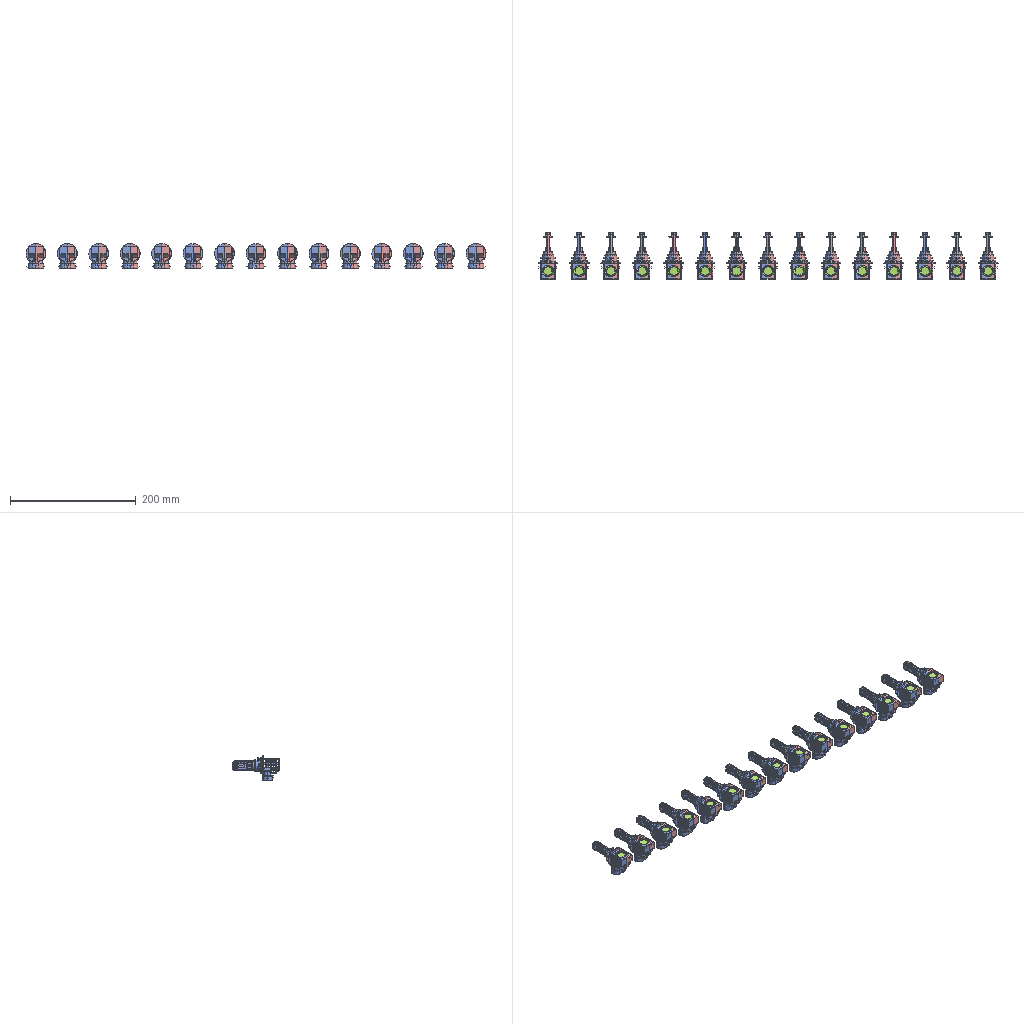Assembly | SolidWorks | 7 different items | 120 placed | box 731 x 74 x 39 mm
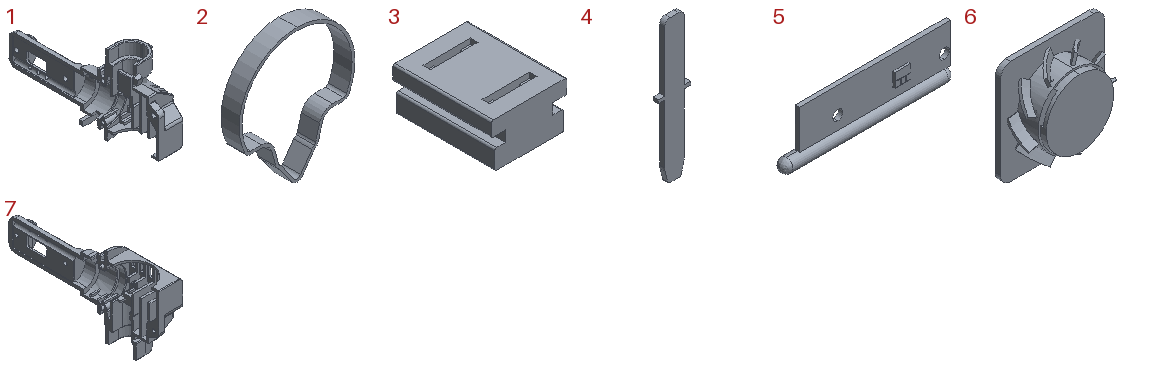Parts list (item | quantity | size | volume | features):
1 | x15 | 19.75 x 73.802 x 39.25 mm | 4726 mm3 | features ICE 12, MoveFace 5, BaseBody 1, Chamfer 1
2 | x15 | 16 x 2.5 x 18.5 mm | 53.347 mm3 | features BaseBody 1
3 | x15 | 7.7 x 10 x 4.6 mm | 286.602 mm3 | features BaseBody 1
4 | x30 | 4.8 x 0.75 x 21 mm | 45.412 mm3 | features BaseBody 1
5 | x15 | 37.94 x 3 x 11.75 mm | 563.627 mm3 | features BaseBody 1
6 | x15 | 20 x 6.3 x 20 mm | 1130 mm3 | features BaseBody 1, ICE 1
7 | x15 | 17.45 x 73.802 x 39.25 mm | 4637 mm3 | features ICE 9, MoveFace 4, BaseBody 1, Chamfer 1, Fillet 1
Mates (type | each side: item.copy, entity, surface, feature):
Coincident | 7.1 face plane Input1 | 1.1 face plane Input1
Concentric | 7.1 face cylinder Input1 | 1.1 face cylinder Input1 | 2 times
Coincident | 7.1 face plane Cut-Extrude1 | 6.1 face plane Input1
Coincident | 1.1 face plane Boss-Extrude1 | 6.1 face plane Boss-Extrude1
Coincident | 1.1 face plane Boss-Extrude2 | 6.1 face plane Boss-Extrude1
Concentric | 1.1 face cylinder Input1 | 2.1 face cylinder Input1
Parallel | 6.1 face plane Boss-Extrude1 | 2.1 face plane Input1
Coincident | 1.1 face plane Input1 | 5.1 face plane Input1
Concentric | 1.1 face cylinder Input1 | 5.1 face cylinder Input1 | 2 times
Coincident | 1.1 face plane Input1 | 3.1 face plane Input1 | 2 times
Parallel | 1.1 face plane Input1 | 3.1 face plane Input1
Coincident | 3.1 face plane Input1 | 4.1 face plane Input1 | 3 times
Coincident | 3.1 face plane Input1 | 4.2 face plane Input1 | 3 times